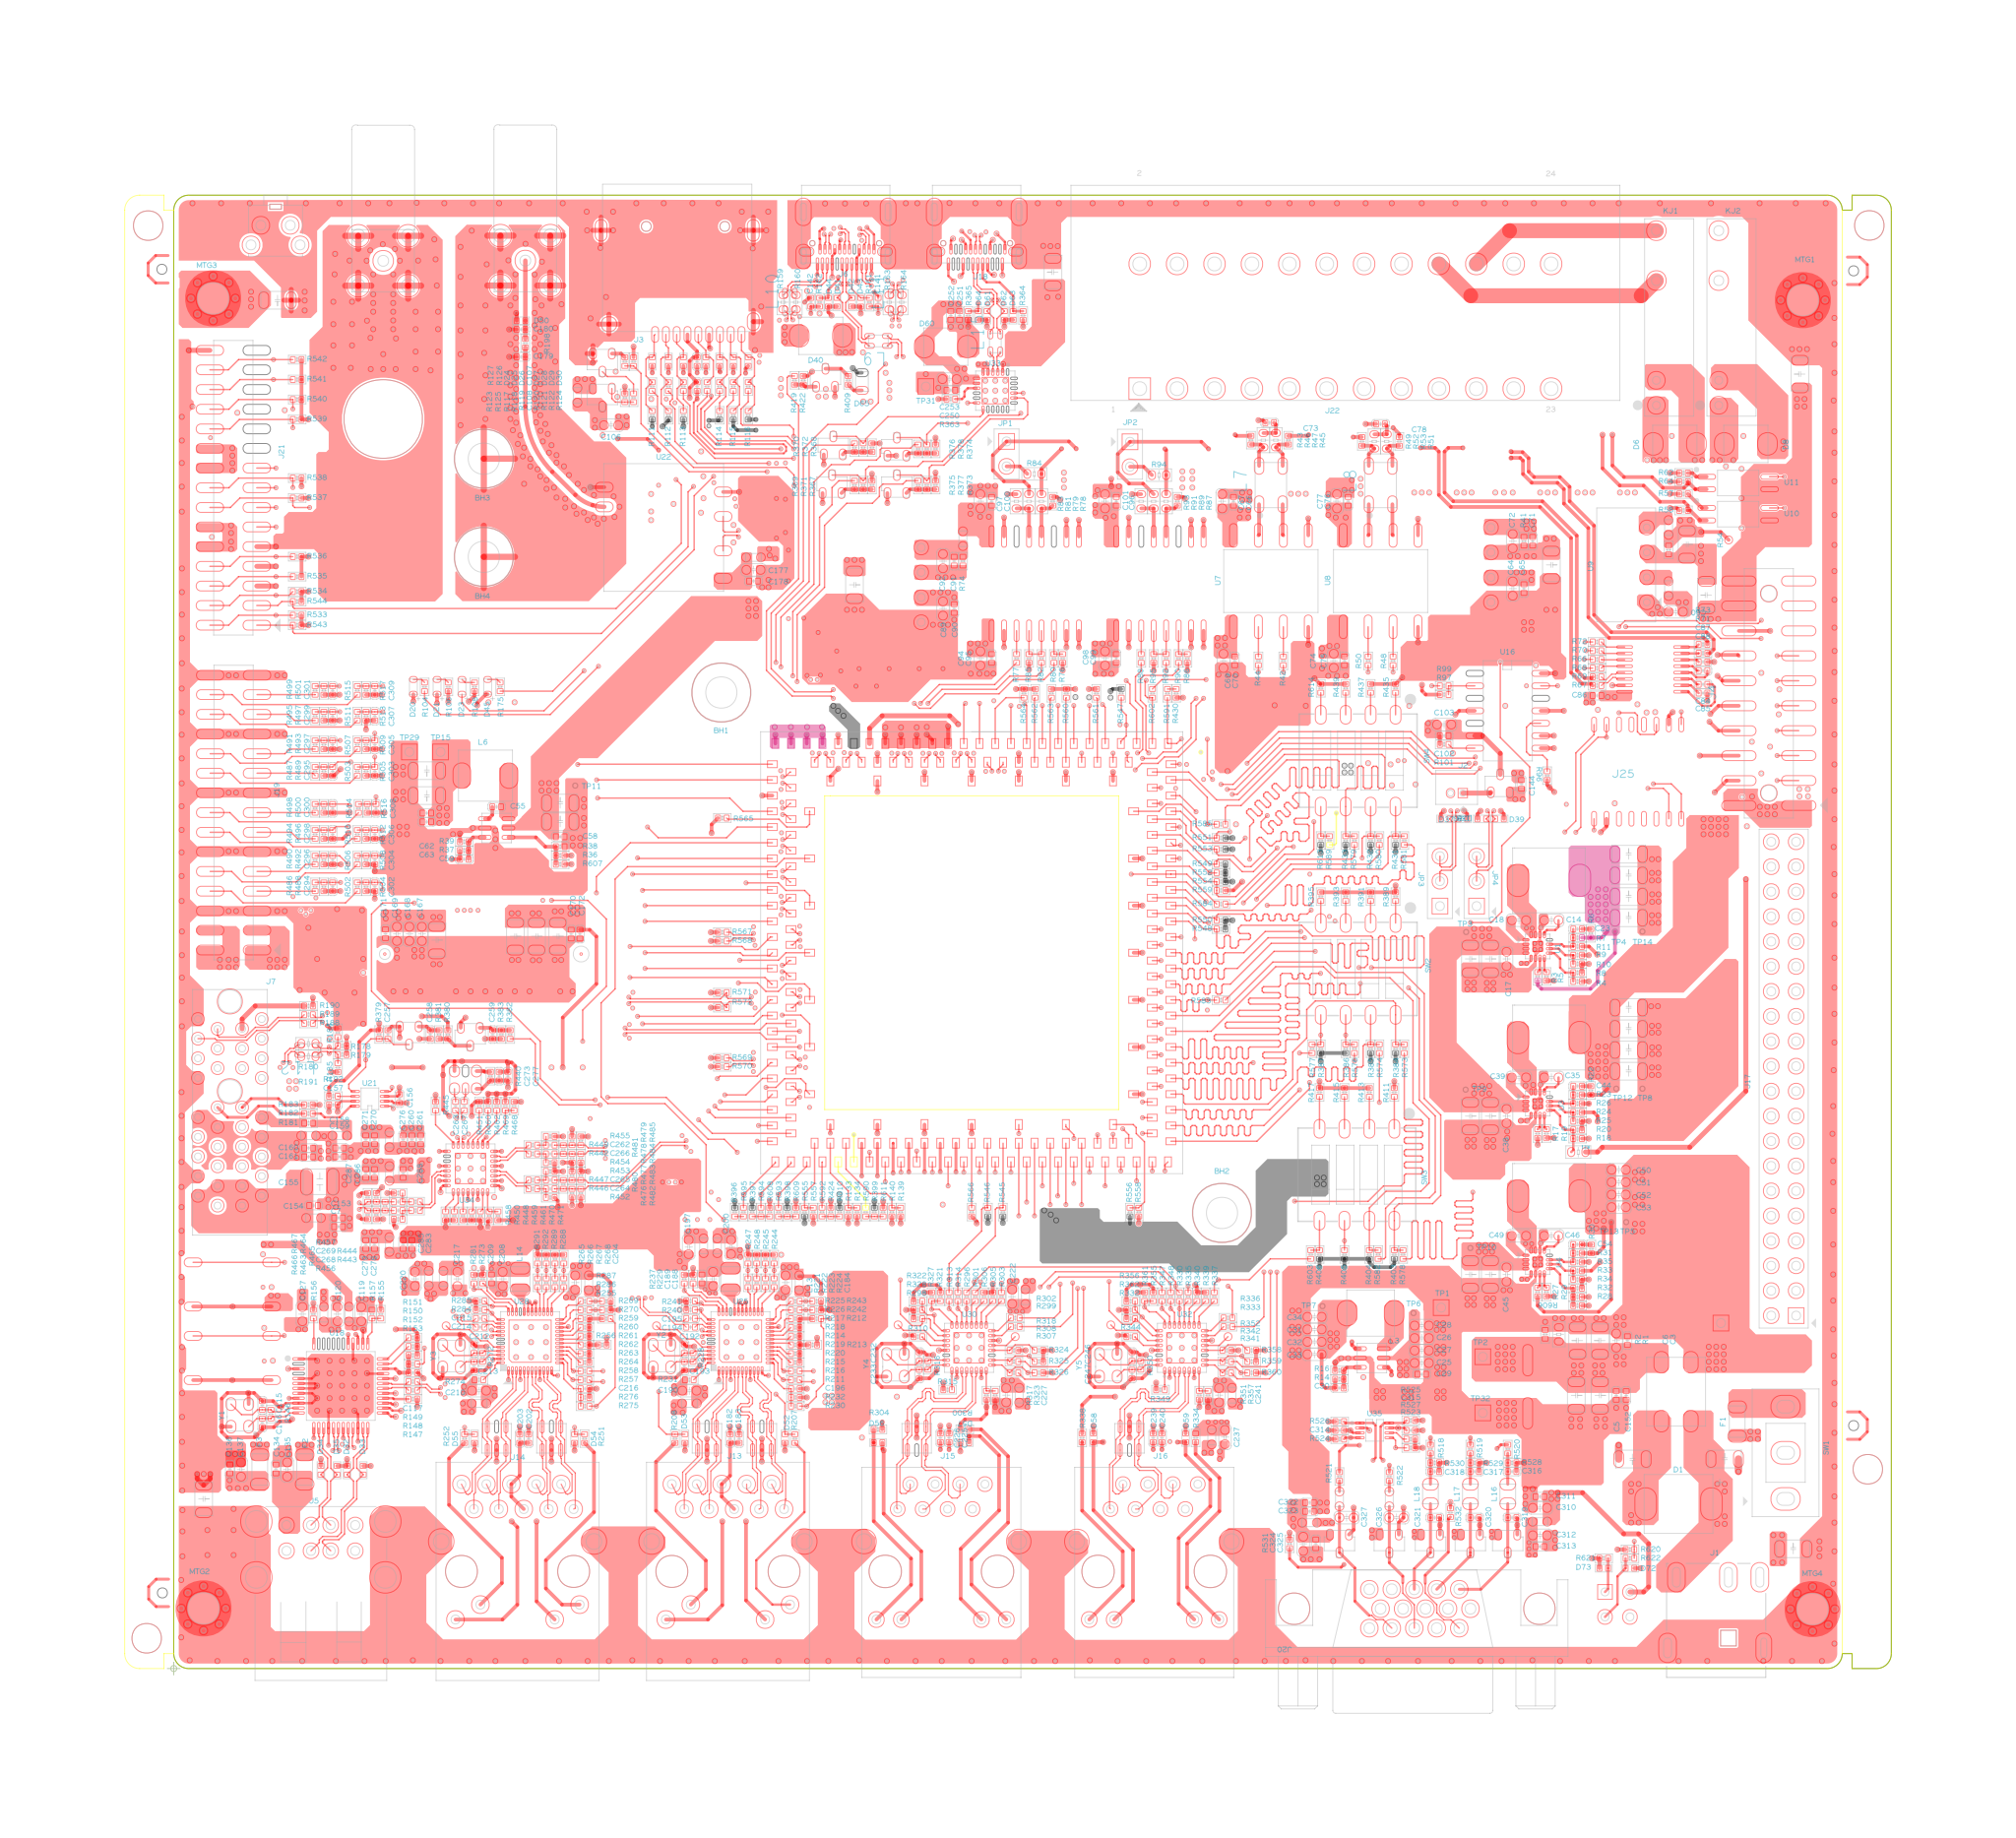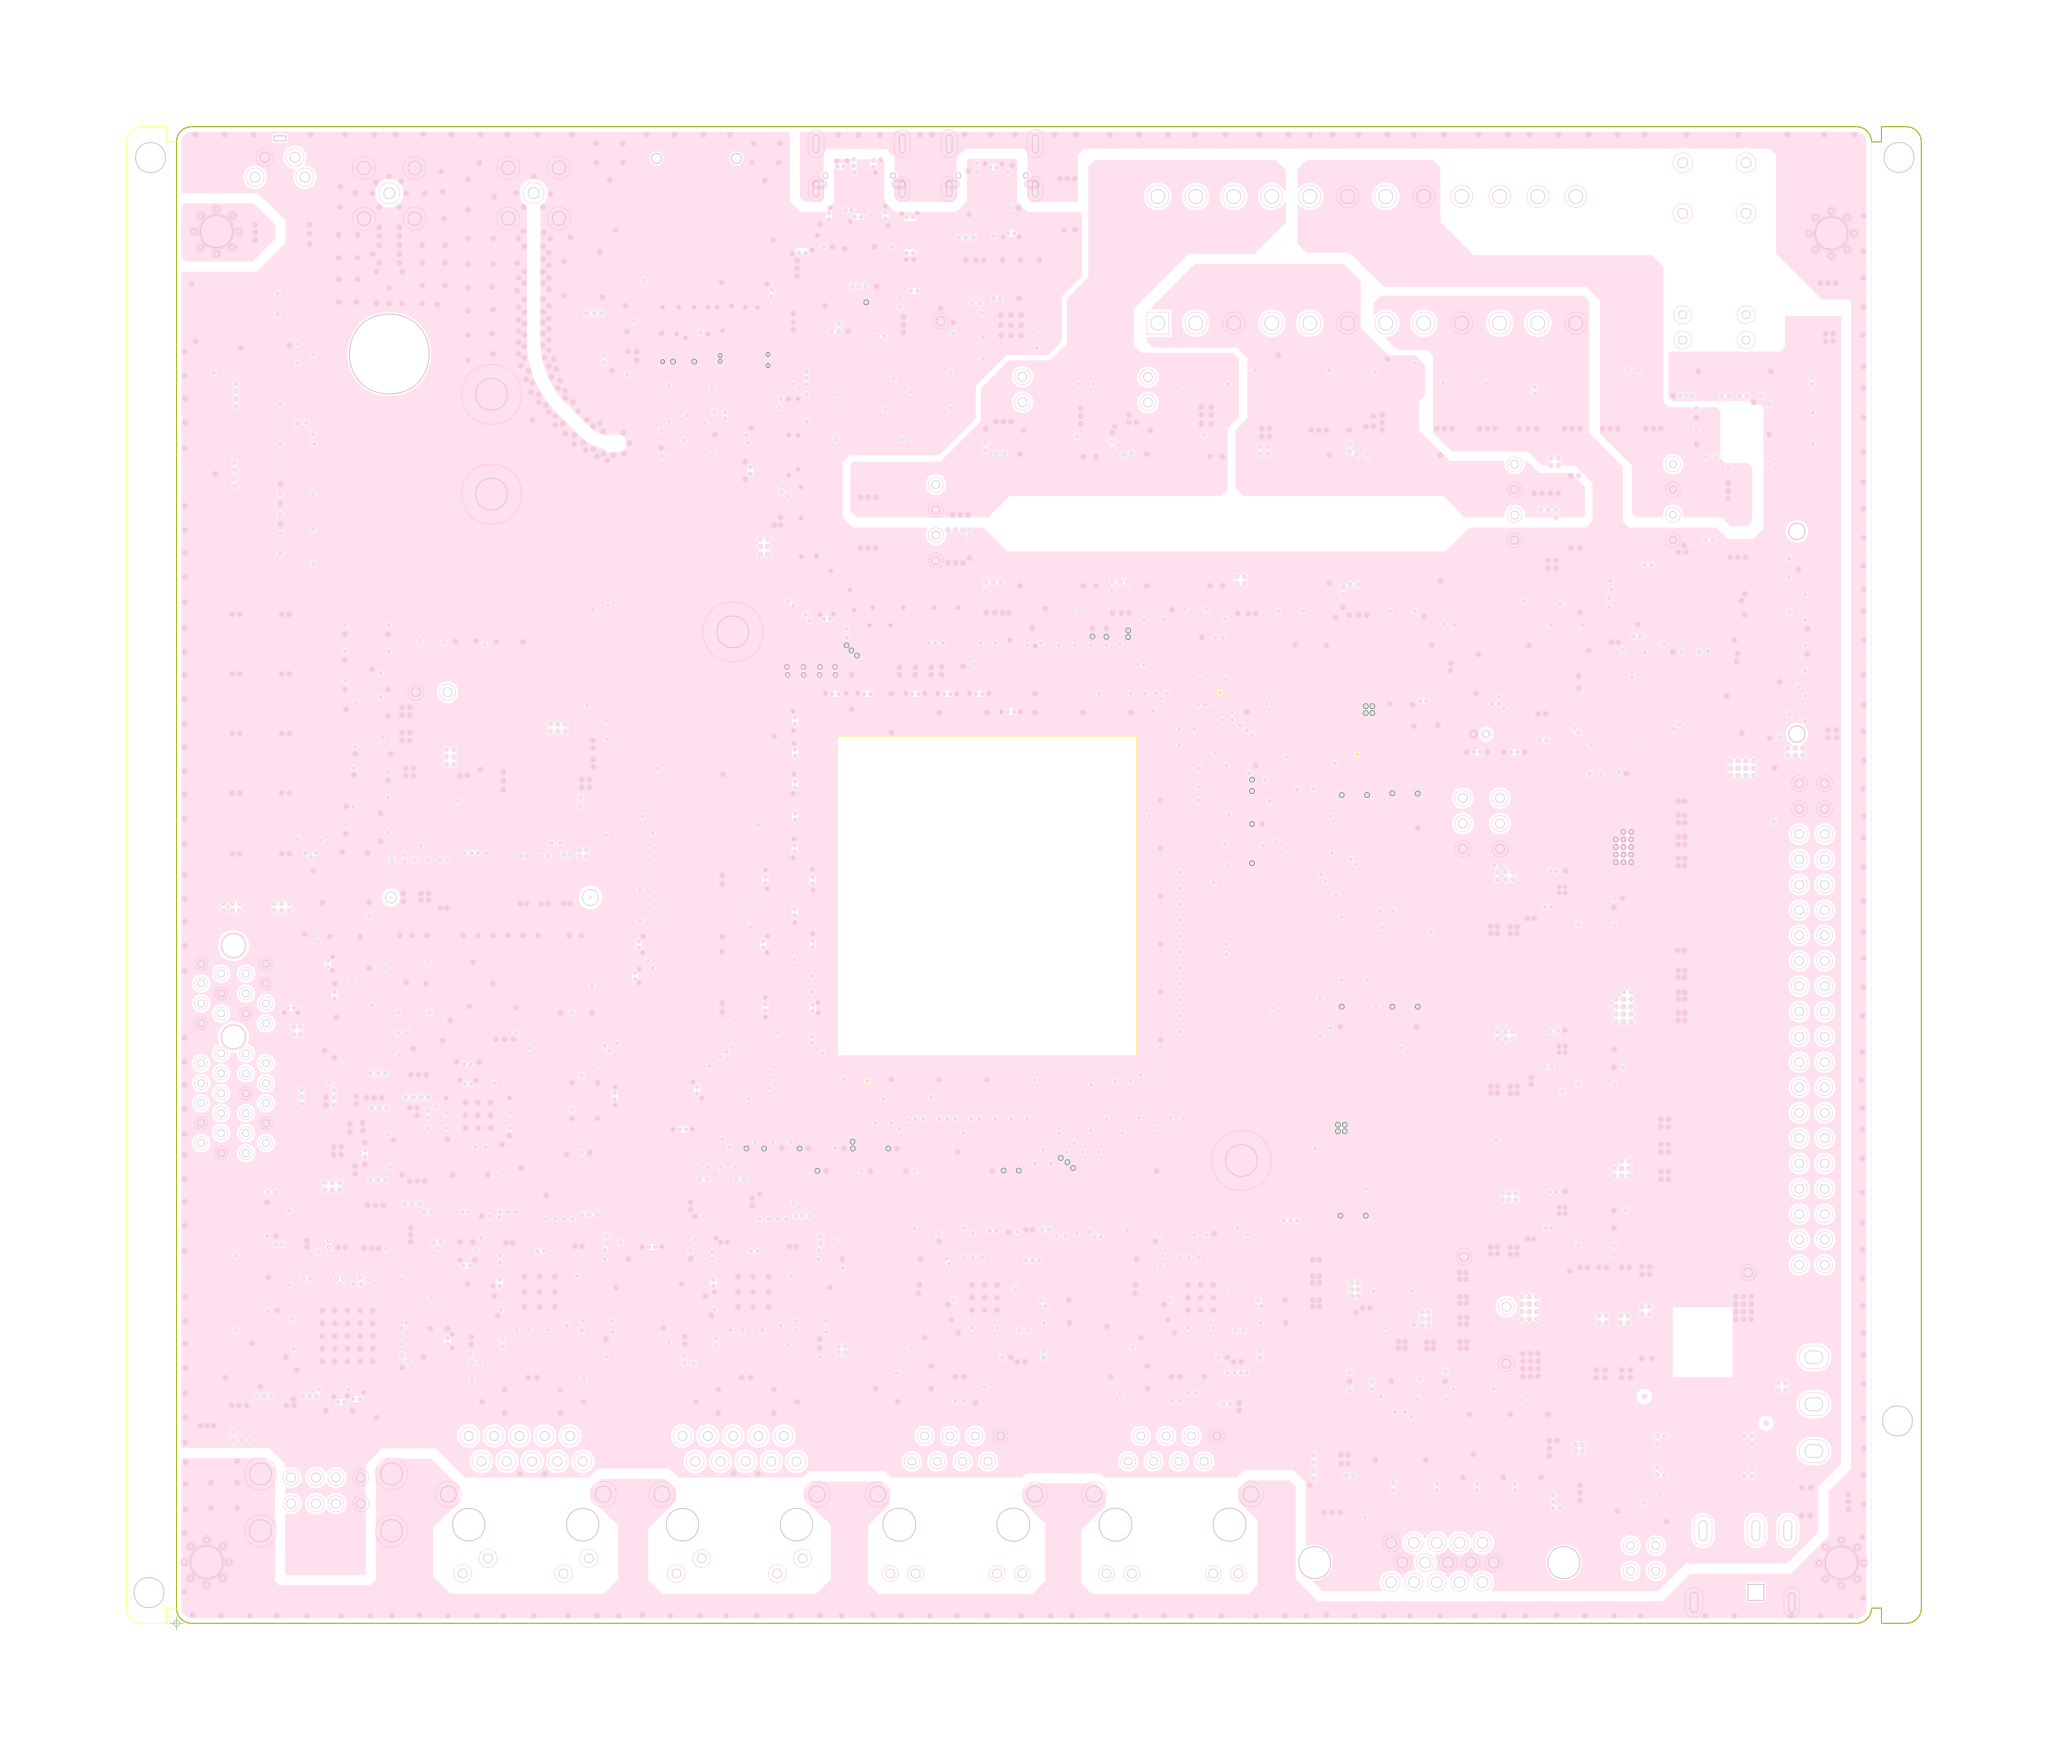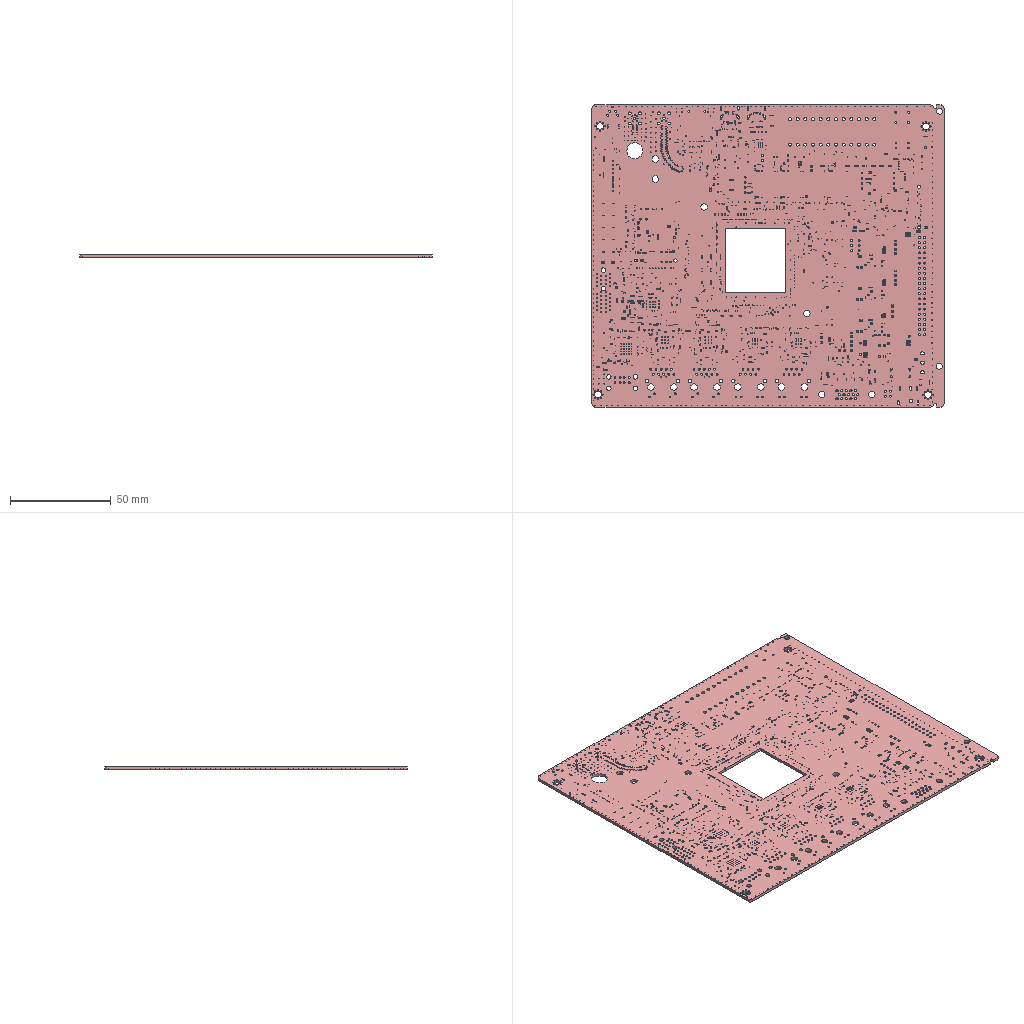Circuit board layout | Cadence Allegro | box 175 x 150 x 1.5 mm
Layer stack:
# Cadence Allegro layer stack of  (unit mm; from the constraint file cross-section; dielectric type: 0 not recorded (Allegro does not mark core vs prepreg), 3 surface material)
index,name,kind,layer,copper_thickness_mm,dielectric_type,dielectric_thickness_mm,dielectric_material,dielectric_constant
0,Top Surface,other,,,,,,
1,TOP,copper,TOP,0.036,,,,
2,Dielectric1,dielectric,,,0,0.0911,FR-4,3.95
3,GND02,copper,GND02,0.03,,,,
4,Dielectric2,dielectric,,,0,0.127,FR-4,3.95
5,ART03,copper,ART03,0.03,,,,
6,Dielectric3,dielectric,,,0,0.927,FR-4,4.5
7,POWER04,copper,POWER04,0.03,,,,
8,Dielectric4,dielectric,,,0,0.127,FR-4,4.5
9,GND05,copper,GND05,0.03,,,,
10,Dielectric5,dielectric,,,0,0.0911,FR-4,4.5
11,BOTTOM,copper,BOTTOM,0.036,,,,
12,Bottom Surface,other,,,,,,
# drill layer pairs: low layer,high layer
drill_pair,TOP,BOTTOM
Part placement, first 442 of 1160 lines:
REFDES,COMP_VALUE,SYM_NAME,SYM_X,SYM_Y,SYM_ROTATE,SYM_MIRROR
BH1,TP,MH236-125T,2196.06,3913.31,0.000,NO
BH2,TP,MH236-125T,4203.94,1826.69,0.000,NO
BH3,TP,MH236-125T,1243.50,4850.83,0.000,NO
BH4,TP,MH236-125T,1243.50,4457.16,0.000,NO
C1,22uF/12/25V,C1206,6035.00,625.00,180.000,YES
C2,22uF/12/25V,C1206,6035.00,715.00,180.000,YES
C3,100nF/4/50V,C0402,5830.00,1315.00,90.000,NO
C4,100uF/6x7/25V,CE6X6,5430.00,1130.00,180.000,NO
C5,100nF/4/50V,C0402,5785.00,1095.00,270.000,NO
C6,1uF/6/25V,C0603,5785.00,1315.00,90.000,NO
C7,100nF/4/50V,C0402,660.71,1771.56,0.000,NO
C8,DNP/C1206,C1206,5720.00,1095.00,270.000,NO
C9,DNP/C1206,C1206,5630.00,1315.00,90.000,NO
C10,22uF/12/25V,C1206,5200.08,2214.92,270.000,NO
C11,22uF/12/25V,C1206,5280.08,2214.92,270.000,NO
C12,DNP/C1206,C1206,5850.00,840.00,180.000,NO
C13,DNP/C1206,C1206,6220.00,840.00,0.000,NO
C14,2.2uF/6/16V,C0603,5525.08,3000.08,0.000,NO
C15,22uF/12/25V,C1206,5625.00,1095.00,270.000,NO
C16,22uF/12/25V,C1206,5720.00,1315.00,90.000,NO
C17,100nF/6/50V,C0603,5345.08,2845.08,270.000,NO
C18,100nF/6/50V,C0603,5395.08,3000.08,0.000,NO
C19,22uF/12/25V,C1206,5835.08,3265.08,0.000,NO
C20,22uF/12/25V,C1206,5835.08,3180.08,0.000,NO
C21,22uF/12/25V,C1206,5835.08,3095.08,0.000,NO
C22,22uF/12/25V,C1206,5835.08,3010.08,0.000,NO
C23,68pF/4/50V,C0402,5630.08,2965.08,180.000,NO
C24,100nF/6/50V,C0603,4805.00,1285.00,180.000,YES
C25,10uF/6/16V,C0603,5005.00,1225.00,0.000,NO
C26,10uF/6/16V,C0603,5005.00,1325.00,0.000,NO
C27,10uF/6/16V,C0603,5005.00,1275.00,0.000,NO
C28,10uF/6/16V,C0603,5005.00,1375.00,0.000,NO
C29,100nF/4/50V,C0402,5005.00,1180.00,0.000,NO
C30,68pF/4/50V,C0402,4675.00,1125.00,0.000,NO
C31,22uF/6/6.3V,C0603,4575.00,1360.00,180.000,NO
C32,22uF/6/6.3V,C0603,4575.00,1310.00,180.000,NO
C33,47uF/6/6.3V,C0603,4575.00,1260.00,180.000,NO
C34,47uF/6/6.3V,C0603,4575.00,1410.00,180.000,NO
C35,2.2uF/6/16V,C0603,5525.08,2369.92,0.000,NO
C36,22uF/12/25V,C1206,5280.08,2845.08,270.000,NO
C37,22uF/12/25V,C1206,5200.08,2845.08,270.000,NO
C38,100nF/6/50V,C0603,5345.08,2214.92,270.000,NO
C39,100nF/6/50V,C0603,5395.08,2369.92,0.000,NO
C40,22uF/12/25V,C1206,5279.92,1579.92,270.000,NO
C41,22uF/12/25V,C1206,5835.08,2479.92,0.000,NO
C42,22uF/12/25V,C1206,5835.08,2394.92,0.000,NO
C43,22uF/12/25V,C1206,5835.08,2649.92,0.000,NO
C44,68pF/4/50V,C0402,5630.08,2334.92,180.000,NO
C45,100nF/6/50V,C0603,5344.92,1579.92,270.000,NO
C46,2.2uF/6/16V,C0603,5524.92,1734.92,0.000,NO
C47,22uF/12/25V,C1206,5199.92,1579.92,270.000,NO
C48,22uF/12/25V,C1206,5835.08,2564.92,0.000,NO
C49,100nF/6/50V,C0603,5394.92,1734.92,0.000,NO
C50,22uF/6/6.3V,C0603,5795.00,2000.00,0.000,NO
C51,22uF/6/6.3V,C0603,5795.00,1950.00,0.000,NO
C52,22uF/6/6.3V,C0603,5795.00,1900.00,0.000,NO
C53,22uF/6/6.3V,C0603,5795.00,1850.00,0.000,NO
C54,68pF/4/50V,C0402,5629.92,1699.92,180.000,NO
C55,100nF/4/50V,C0402,1295.00,3455.00,0.000,NO
C56,22uF/12/25V,C1206,1550.00,3470.00,0.000,NO
C57,22uF/12/25V,C1206,1550.00,3395.00,0.000,NO
C58,100nF/4/50V,C0402,1550.00,3335.00,0.000,NO
C59,1uF/4/50V,C0402,1165.00,3245.00,0.000,NO
C60,DNP,C1206,1015.00,3500.00,180.000,NO
C61,22uF/12/25V,C1206,1015.00,3600.00,180.000,NO
C62,100nF/4/50V,C0402,1015.00,3430.00,180.000,NO
C63,100nF/4/50V,C0402,1015.00,3395.00,180.000,NO
C64,10uF/6/16V,C0603,5370.00,4329.95,270.000,NO
C65,100nF/4/50V,C0402,5415.00,4329.95,270.000,NO
C66,100nF/4/50V,C0402,4250.00,4680.00,90.000,NO
C67,10uF/6/16V,C0603,4205.00,4680.00,90.000,NO
C68,DNP/C1206,C1206,5525.00,4424.95,270.000,NO
C69,10uF/6/10V,C0603,4210.00,4040.00,270.000,NO
C70,100nF/4/50V,C0402,4255.00,4040.00,270.000,NO
C71,100nF/4/50V,C0402,5450.00,4519.95,270.000,NO
C72,10uF/6/10V,C0603,5370.00,4519.95,270.000,NO
C73,68pF/4/50V,C0402,4395.00,4995.00,180.000,NO
C74,10uF/6/10V,C0603,4652.24,4040.41,270.000,NO
C75,100nF/4/50V,C0402,4695.00,4040.00,270.000,NO
C76,100nF/4/50V,C0402,4710.00,4680.00,90.000,NO
C77,10uF/6/10V,C0603,4665.00,4680.00,90.000,NO
C78,68pF/4/50V,C0402,4840.00,4990.00,180.000,NO
C79,22uF/12/25V,C1206,6069.00,4507.00,270.000,NO
C80,10uF/6/16V,C0603,6024.00,4237.00,180.000,NO
C81,DNP/C1206,C1206,6147.00,4304.00,90.000,NO
C82,10nF/4/50V,C0402,6305.00,4657.69,0.000,YES
C83,10nF/4/50V,C0402,6305.00,4732.31,0.000,YES
C84,100nF/4/50V,C0402,6133.00,3946.00,180.000,NO
C85,100nF/4/50V,C0402,6133.00,3911.00,180.000,NO
C86,100nF/4/50V,C0402,5708.00,3901.00,180.000,NO
C87,100nF/4/50V,C0402,6133.00,4036.00,180.000,NO
C88,100nF/4/50V,C0402,6133.00,4001.00,180.000,NO
C89,10uF/6/16V,C0603,3085.00,4249.95,270.000,NO
C90,100nF/4/50V,C0402,3130.00,4249.95,270.000,NO
C91,100nF/4/50V,C0402,3130.00,4439.95,270.000,NO
C92,10uF/6/16V,C0603,3085.00,4439.95,270.000,NO
C93,DNP/C1206,C1206,2730.00,4344.95,270.000,NO
C94,10uF/6/16V,C0603,3235.00,4050.00,270.000,NO
C95,100nF/4/50V,C0402,3280.00,4050.00,270.000,NO
C96,100nF/4/50V,C0402,3780.00,4680.00,90.000,NO
C97,10uF/6/16V,C0603,3235.00,4680.00,90.000,NO
C98,10uF/6/16V,C0603,3735.00,4050.00,270.000,NO
C99,100nF/4/50V,C0402,3780.00,4050.00,270.000,NO
C100,100nF/4/50V,C0402,3280.00,4680.00,90.000,NO
C101,10uF/6/16V,C0603,3735.00,4680.00,90.000,NO
C102,100nF/4/50V,C0402,5095.00,3740.00,180.000,NO
C103,10uF/6/16V,C0603,5095.00,3785.00,180.000,NO
C104,100nF/4/50V,C0402,375.00,1560.00,180.000,YES
C105,100nF/4/50V,C0402,380.00,1265.00,180.000,YES
C106,10uF/6/16V,C0603,1754.00,4985.00,0.000,NO
C107,1uF/4/6.3V,C0402,2099.00,5240.00,270.000,NO
C108,100nF/4/50V,C0402,2099.00,5140.00,270.000,NO
C109,10uF/6/16V,C0603,6495.96,3457.99,180.000,YES
C110,100nF/4/50V,C0402,6307.04,3458.01,0.000,YES
C111,18pF/4/50V,C0402,6401.99,3843.04,90.000,YES
C112,18pF/4/50V,C0402,6401.99,3943.04,90.000,YES
C113,18pF/4/50V,C0402,6366.99,3743.04,90.000,YES
C114,100nF/4/50V,C0402,5924.00,3801.00,0.000,YES
C115,DNP,C0402,355.00,1055.00,90.000,NO
C116,DNP,C0402,355.00,985.00,270.000,NO
C117,DNP,C0402,959.00,1186.00,0.000,NO
C118,100nF/4/50V,C0402,775.00,1295.00,90.000,YES
C119,10uF/6/10V,C0603,752.00,1421.00,90.000,NO
C120,10uF/6/10V,C0603,657.00,1421.00,90.000,NO
C121,100nF/4/50V,C0402,560.00,975.00,270.000,YES
C122,100nF/4/50V,C0402,680.00,970.00,270.000,YES
C123,100nF/4/50V,C0402,835.00,1065.00,0.000,YES
C124,100nF/4/50V,C0402,835.00,1165.00,0.000,YES
C125,100nF/4/50V,C0402,700.00,1295.00,90.000,YES
C126,100nF/4/50V,C0402,740.00,1295.00,90.000,YES
C127,10uF/6/10V,C0603,516.00,1421.00,90.000,NO
C128,100nF/4/50V,C0402,835.00,1100.00,0.000,YES
C129,100nF/4/50V,C0402,505.00,1165.00,180.000,YES
C130,100nF/4/50V,C0402,835.00,1030.00,0.000,YES
C131,100nF/4/50V,C0402,510.00,1085.00,180.000,YES
C132,100nF/4/50V,C0402,505.00,1200.00,180.000,YES
C133,100nF/4/50V,C0402,510.00,1050.00,180.000,YES
C134,100nF/4/50V,C0402,410.00,800.00,90.000,NO
C135,10uF/6/10V,C0603,455.00,798.00,90.000,NO
C136,100nF/4/50V,C0402,225.00,800.00,90.000,NO
C137,10uF/6/10V,C0603,270.00,798.00,90.000,NO
C139,100nF/4/50V,C0402,2625.00,5478.13,90.000,YES
C140,10pF/4/50V,C0402,2555.00,5478.13,90.000,YES
C141,1nF/4/50V,C0402,2825.00,5478.13,90.000,NO
C142,1nF/4/50V,C0402,2555.00,5478.13,90.000,NO
C144,100nF/4/50V,C0402,5405.00,3545.00,90.000,NO
C145,100nF/4/50V,C0402,2590.00,5478.13,90.000,YES
C146,10uF/6/16V,C0603,2809.88,5115.00,180.000,YES
C147,100nF/4/50V,C0402,2809.88,5160.00,180.000,YES
C148,4.7uF/6/16V,C0603,2509.88,5155.00,0.000,YES
C149,100nF/4/50V,C0402,2755.00,5478.13,90.000,YES
C150,100nF/4/50V,C0402,2790.00,5478.13,90.000,YES
C151,10uF/6/16V,C0603,2509.88,5105.00,0.000,YES
C152,100nF/4/50V,C0402,5825.00,1095.00,270.000,NO
C153,100nF/4/50V,C0402,660.71,1806.56,0.000,NO
C154,100nF/4/50V,C0402,560.71,1856.56,0.000,NO
C155,10uF/1210/50V,C1210,585.71,1951.56,0.000,NO
C156,100nF/4/50V,C0402,905.00,2285.00,270.000,NO
C157,100nF/4/50V,C0402,640.00,2260.00,180.000,NO
C158,100nF/4/50V,C0402,665.00,2087.00,0.000,NO
C159,100nF/4/50V,C0402,665.00,2052.00,0.000,NO
C160,100nF/4/50V,C0402,540.71,2086.56,0.000,NO
C161,100nF/4/50V,C0402,540.71,2051.56,0.000,NO
C162,33pF/4/50V,C0402,1720.00,5020.00,90.000,YES
C163,100nF/4/50V,C0402,1720.00,5140.00,90.000,YES
C164,100uF/12/6.3V,C1206,1455.00,2935.64,270.000,NO
C165,100uF/12/6.3V,C1206,1540.00,2935.64,270.000,NO
C166,100uF/12/6.3V,C1206,1370.00,2935.64,270.000,NO
C167,10uF/6/16V,C0603,995.00,2945.64,270.000,NO
C168,10uF/6/16V,C0603,945.00,2945.64,270.000,NO
C169,1uF/6/16V,C0603,895.00,2945.64,270.000,NO
C170,100nF/4/50V,C0402,1594.00,2944.64,270.000,NO
C171,33pF/4/50V,C0402,849.00,2946.00,270.000,NO
C172,10nF/4/50V,C0402,1629.00,2944.64,270.000,NO
C173,33pF/4/50V,C0402,1910.00,5030.00,270.000,YES
C174,33pF/4/50V,C0402,2020.00,5030.00,270.000,YES
C175,33pF/4/50V,C0402,1975.00,5030.00,270.000,YES
C176,100uF/12/6.3V,C1206,1055.00,2920.64,270.000,NO
C177,10uF/6/16V,C0603,2325.00,4405.00,0.000,NO
C178,100nF/4/50V,C0402,2325.00,4360.00,0.000,NO
C179,DNP,C0402,1392.68,5259.00,180.000,NO
C180,DNP,C0402,1392.68,5369.00,180.000,NO
C181,10nF/4/50V,C0402,1515.00,2455.00,90.000,YES
C182,100nF/4/50V,C0402,2231.13,922.00,90.000,NO
C183,100nF/4/50V,C0402,2267.13,922.00,90.000,NO
C184,4.7uF/6/16V,C0603,2453.74,1547.61,270.000,NO
C185,100nF/4/50V,C0402,2245.13,1431.00,0.000,YES
C186,100nF/4/50V,C0402,2316.13,1431.00,180.000,YES
C188,4.7uF/6/16V,C0603,2163.13,1562.00,270.000,NO
C189,100nF/4/50V,C0402,2118.13,1562.00,270.000,NO
C190,10uF/6/16V,C0603,2068.13,1114.00,180.000,NO
C191,100nF/4/50V,C0402,2202.13,1195.00,180.000,YES
C192,33pF/4/50V,C0402,2047.74,1282.61,90.000,NO
C193,33pF/4/50V,C0402,2047.74,1212.61,270.000,NO
C194,10nF/4/50V,C0402,2072.74,1368.61,0.000,NO
C195,10nF/4/50V,C0402,2072.74,1403.61,0.000,NO
C196,100nF/4/50V,C0402,2493.13,1122.00,0.000,NO
C197,4.7uF/6/16V,C0603,2065.00,1690.00,270.000,NO
C198,100nF/4/50V,C0402,2272.13,1195.00,180.000,YES
C199,100nF/4/50V,C0402,2156.13,1242.00,270.000,YES
C200,10uF/6/16V,C0603,2235.00,1690.00,270.000,NO
C201,100nF/4/50V,C0402,2392.13,1351.00,90.000,YES
C202,100nF/4/50V,C0402,1423.33,922.00,90.000,NO
C203,100nF/4/50V,C0402,1387.33,922.00,90.000,NO
C204,4.7uF/6/16V,C0603,1609.94,1547.61,270.000,NO
C205,100nF/4/50V,C0402,1401.33,1431.00,0.000,YES
C206,100nF/4/50V,C0402,1472.33,1431.00,180.000,YES
C208,4.7uF/6/16V,C0603,1319.33,1562.00,270.000,NO
C209,100nF/4/50V,C0402,1274.33,1562.00,270.000,NO
C210,10uF/6/16V,C0603,1224.33,1114.00,180.000,NO
C211,100nF/4/50V,C0402,1358.33,1195.00,180.000,YES
C212,33pF/4/50V,C0402,1203.94,1282.61,90.000,NO
C213,33pF/4/50V,C0402,1203.94,1212.61,270.000,NO
C214,10nF/4/50V,C0402,1228.94,1368.61,0.000,NO
C215,10nF/4/50V,C0402,1228.94,1403.61,0.000,NO
C216,100nF/4/50V,C0402,1649.33,1122.00,0.000,NO
C217,4.7uF/6/16V,C0603,1137.54,1562.00,270.000,NO
C218,100nF/4/50V,C0402,1310.89,1240.11,270.000,YES
C219,100nF/4/50V,C0402,1428.33,1195.00,180.000,YES
C220,10uF/6/16V,C0603,967.54,1562.00,270.000,NO
C221,100nF/4/50V,C0402,1548.33,1351.00,90.000,YES
C222,10uF/6/16V,C0603,3362.57,1490.80,90.000,NO
C223,100nF/4/50V,C0402,3280.57,1296.80,90.000,YES
C224,100nF/4/50V,C0402,3249.57,1490.80,270.000,YES
C225,100nF/4/50V,C0402,3109.57,925.00,90.000,NO
C226,100nF/4/50V,C0402,3074.57,925.00,90.000,NO
C227,10uF/6/16V,C0603,3338.57,1095.80,270.000,NO
C228,100nF/4/50V,C0402,3257.57,1193.80,180.000,YES
C230,1uF/4/6.3V,C0402,3187.57,1193.80,180.000,YES
C231,100nF/4/50V,C0402,3117.57,1193.80,0.000,YES
C232,33pF/4/50V,C0402,2989.57,1250.80,90.000,NO
C233,33pF/4/50V,C0402,2989.57,1180.80,270.000,NO
C234,1uF/4/6.3V,C0402,3098.57,1256.80,90.000,YES
C235,100nF/4/50V,C0402,3098.57,1326.80,270.000,YES
C236,100nF/4/50V,C0402,4103.11,1490.80,270.000,YES
C237,10uF/6/16V,C0603,4215.89,928.20,270.000,NO
C238,100nF/4/50V,C0402,4134.11,1296.80,90.000,YES
C239,100nF/4/50V,C0402,3928.11,925.00,90.000,NO
C240,100nF/4/50V,C0402,3963.11,925.00,90.000,NO
C241,10uF/6/16V,C0603,4192.11,1095.80,270.000,NO
C242,100nF/4/50V,C0402,4111.11,1193.80,180.000,YES
C244,1uF/4/6.3V,C0402,4041.11,1193.80,180.000,YES
C245,100nF/4/50V,C0402,3971.11,1193.80,0.000,YES
C246,33pF/4/50V,C0402,3843.11,1250.80,90.000,NO
C247,33pF/4/50V,C0402,3843.11,1180.80,270.000,NO
C248,1uF/4/6.3V,C0402,3952.11,1256.80,90.000,YES
C249,100nF/4/50V,C0402,3952.11,1326.80,270.000,YES
C250,100nF/4/50V,C0402,3116.33,5125.00,180.000,NO
C251,10pF/4/50V,C0402,3151.33,5425.00,270.000,NO
C252,100nF/4/50V,C0402,3116.33,5425.00,270.000,NO
C253,10uF/6/16V,C0603,3111.33,5170.00,180.000,NO
C254,DNP,C0603,3220.17,5150.00,90.000,YES
C255,100nF/4/50V,C0402,3280.17,5200.00,180.000,YES
C256,0,C1206,3526.00,5599.00,90.000,NO
C257,100nF/4/50V,C0402,859.00,2542.00,90.000,NO
C258,100nF/4/50V,C0402,1029.00,2542.00,270.000,NO
C259,10nF/4/50V,C0402,1279.00,2542.00,270.000,NO
C260,10uF/6/16V,C0402,955.00,2120.00,90.000,NO
C261,100nF/4/50V,C0402,990.00,2120.00,90.000,NO
C262,100nF/4/50V,C0402,1510.00,2098.45,180.000,NO
C263,100nF/4/50V,C0402,1130.00,2255.00,270.000,NO
C264,100nF/4/50V,C0402,1510.00,1923.45,180.000,NO
C265,100nF/4/50V,C0402,1510.00,1958.45,180.000,NO
C266,100nF/4/50V,C0402,1510.00,2063.45,180.000,NO
C267,100nF/4/50V,C0402,1165.00,2255.00,270.000,NO
C268,100nF/4/50V,C0402,900.00,1836.43,0.000,NO
C269,100nF/4/50V,C0402,900.00,1871.43,0.000,NO
C270,10uF/4/6.3V,C0402,805.00,2120.00,270.000,NO
C271,100nF/4/50V,C0402,770.00,2120.00,270.000,NO
C272,100nF/4/50V,C0402,920.00,2120.00,270.000,YES
C273,10uF/4/6.3V,C0402,1305.00,2375.00,90.000,NO
C274,10uF/4/6.3V,C0402,990.00,2120.00,270.000,YES
C275,100nF/4/50V,C0402,955.00,2120.00,270.000,YES
C276,100nF/4/50V,C0402,920.00,2120.00,90.000,NO
C277,100nF/4/50V,C0402,1340.00,2375.00,90.000,NO
C278,10uF/4/6.3V,C0402,805.00,1700.00,270.000,NO
C279,100nF/4/50V,C0402,770.00,1700.00,270.000,NO
C280,100nF/4/50V,C0402,1220.00,2100.00,0.000,YES
C281,10uF/4/6.3V,C0402,920.00,1700.00,270.000,YES
C282,10uF/4/6.3V,C0402,1155.00,1910.00,0.000,YES
C283,100nF/4/50V,C0402,955.00,1700.00,90.000,NO
C284,100nF/4/50V,C0402,955.00,1700.00,270.000,YES
C285,100nF/4/50V,C0402,920.00,1700.00,90.000,NO
C286,10uF/4/6.3V,C0402,805.00,1985.00,270.000,NO
C287,100nF/4/50V,C0402,770.00,1985.00,270.000,NO
C288,100nF/4/50V,C0402,920.00,1985.00,90.000,NO
C289,10uF/4/6.3V,C0402,1240.00,1910.00,180.000,YES
C290,10uF/4/6.3V,C0402,1285.00,2050.00,270.000,YES
C291,100nF/4/50V,C0402,1095.00,2040.00,270.000,YES
C292,100nF/4/50V,C0402,1095.00,1945.00,90.000,YES
C293,100nF/4/50V,C0402,1285.00,1960.00,90.000,YES
C294,10nF/4/50V,C0402,637.10,3134.47,270.000,NO
C295,10nF/4/50V,C0402,637.10,3597.47,270.000,NO
C296,10nF/4/50V,C0402,637.10,3241.47,270.000,NO
C297,10nF/4/50V,C0402,637.10,3703.69,270.000,NO
C298,10nF/4/50V,C0402,637.10,3344.47,270.000,NO
C299,10nF/4/50V,C0402,637.10,3818.69,270.000,NO
C300,10nF/4/50V,C0402,637.10,3448.69,270.000,NO
C301,10nF/4/50V,C0402,637.10,3921.69,270.000,NO
C302,10nF/4/50V,C0402,806.10,3134.47,270.000,NO
C303,10nF/4/50V,C0402,806.10,3597.47,270.000,NO
C304,10nF/4/50V,C0402,806.10,3241.47,270.000,NO
C305,10nF/4/50V,C0402,806.10,3703.69,270.000,NO
C306,10nF/4/50V,C0402,806.10,3344.47,270.000,NO
C307,10nF/4/50V,C0402,806.10,3818.69,270.000,NO
C308,10nF/4/50V,C0402,811.10,3448.69,270.000,NO
C309,10nF/4/50V,C0402,806.10,3921.69,270.000,NO
C310,10uF/6/16V,C0603,5479.00,644.00,180.000,NO
C311,100nF/4/50V,C0402,5479.00,689.00,180.000,NO
C312,10uF/6/16V,C0603,5479.00,534.00,0.000,NO
C313,100nF/4/50V,C0402,5479.00,489.00,0.000,NO
C314,100nF/4/50V,C0402,4676.00,955.00,180.000,NO
C315,100nF/4/50V,C0402,4961.00,955.00,0.000,NO
C316,10pF/4/50V,C0402,5367.32,790.00,0.000,NO
C317,10pF/4/50V,C0402,5217.32,790.00,0.000,NO
C318,10pF/4/50V,C0402,5057.32,790.00,0.000,NO
C319,10pF/4/50V,C0402,5367.32,605.00,0.000,NO
C320,10pF/4/50V,C0402,5217.32,605.00,0.000,NO
C321,10pF/4/50V,C0402,5057.32,605.00,0.000,NO
C322,10uF/6/16V,C0402,4555.00,665.00,0.000,NO
C323,100nF/4/50V,C0402,4555.00,630.00,0.000,NO
C324,10uF/6/16V,C0603,4530.00,500.00,270.000,NO
C325,100nF/4/50V,C0402,4580.00,500.00,270.000,NO
C326,470pF/6/50V,C0603,4903.51,605.00,0.000,NO
C327,470pF/6/50V,C0603,4703.51,605.00,0.000,NO
C328,0,C1206,416.00,5486.00,180.000,NO
C329,0,C1206,6522.00,5190.00,90.000,NO
C330,0,C1206,6495.00,480.00,0.000,NO
C331,0,C1206,120.00,680.00,270.000,NO
C332,100nF/4/50V,C0402,2390.00,1245.00,270.000,YES
C333,100nF/4/50V,C0402,2345.00,1195.00,180.000,YES
C334,100nF/4/50V,C0402,1545.00,1247.00,270.000,YES
C335,100nF/4/50V,C0402,1500.00,1195.00,180.000,YES
C336,100nF/4/50V,C0402,390.00,5080.00,180.000,YES
D1,SMCJ15CA,DO-214AB,6035.00,660.00,180.000,NO
D2,SMBJ15CA,DO-214AA,4320.00,4860.00,270.000,YES
D3,SMBJ15CA,DO-214AA,4490.00,4860.00,270.000,YES
D4,SMBJ15CA,DO-214AA,4660.00,4860.00,270.000,YES
D5,SMBJ15CA,DO-214AA,4830.00,4860.00,270.000,YES
D6,PMEG4030EP,DO-214AA,6020.00,4910.00,180.000,NO
D7,SMBJ12CA,DO-214AA,5665.00,4860.00,270.000,YES
D8,PMEG4030EP,DO-214AA,6305.00,4910.00,180.000,NO
D9,SMBJ12CA,DO-214AA,5830.00,4860.00,270.000,YES
D10,SMBJ15CA,DO-214AA,5000.00,4860.00,270.000,YES
D11,SMBJ15CA,DO-214AA,5170.00,4860.00,270.000,YES
D12,SMBJ15CA,DO-214AA,5335.00,4860.00,270.000,YES
D13,SMBJ15CA,DO-214AA,5500.00,4860.00,270.000,YES
D14,SMBJ12CA,DO-214AA,3505.00,4860.00,270.000,YES
D15,SMBJ12CA,DO-214AA,3675.00,4860.00,270.000,YES
D16,SMBJ12CA,DO-214AA,3980.00,4860.00,270.000,YES
D17,SMBJ12CA,DO-214AA,4150.00,4860.00,270.000,YES
D18,LBAT54CLT1G,SOT-23,5320.00,3550.00,0.000,NO
D20,LED-SML1206,LED0603,960.97,3936.00,90.000,NO
D21,LED-SML1206,LED0603,1055.97,3936.00,90.000,NO
D23,LED-SML1206,LED0603,1155.97,3936.00,90.000,NO
D24,B72590D50H160,D0402,1919.00,5240.00,90.000,NO
D25,B72590D50H160,D0402,1984.00,5240.00,90.000,NO
D26,B72590D50H160,D0402,2044.00,5240.00,90.000,NO
D27,B72590D50H160,D0402,2134.00,5240.00,90.000,NO
D28,B72590D50H160,D0402,2189.00,5240.00,90.000,NO
D29,B72590D50H160,D0402,2244.00,5240.00,90.000,NO
D30,B72590D50H160,D0402,2304.00,5240.00,90.000,NO
D32,B72590D50H160,D0402,695.00,795.00,270.000,NO
D33,B72590D50H160,D0402,760.00,795.00,270.000,NO
D34,B72590D50H160,D0402,590.00,795.00,270.000,NO
D35,B72590D50H160,D0402,655.00,795.00,270.000,NO
D36,B72590D50H160,D0402,5099.02,3406.60,0.000,NO
D37,B72590D50H160,D0402,5169.88,3406.60,180.000,NO
D38,B72590D50H160,D0402,5246.02,3406.60,0.000,NO
D39,B72590D50H160,D0402,5316.88,3406.60,180.000,NO
D40,SMBJ6.0CA,DO-214AA,2595.00,5343.13,0.000,NO
D41,B72590D50H160,D0402,2659.88,5478.13,90.000,NO
D42,B72590D50H160,D0402,2719.88,5478.13,90.000,NO
D43,B72590D50H160,D0402,2755.00,5478.13,90.000,NO
D44,B72590D50H160,D0402,2625.00,5478.13,90.000,NO
D45,LED-SML1206,LED0603,1259.00,3936.00,90.000,NO
D46,B72590D50H160,D0402,1755.00,5140.00,270.000,YES
D47,B72590D50H160,D0402,1910.00,5140.00,270.000,YES
D48,B72590D50H160,D0402,2020.00,5140.00,270.000,YES
D49,B72590D50H160,D0402,1975.00,5140.00,270.000,YES
D50,DNP,D0402,1392.68,5404.00,0.000,NO
D51,B72590D50H160,D0402,822.68,5404.00,180.000,YES
D52,B72590D50H160,D0402,2451.13,922.00,90.000,NO
D53,B72590D50H160,D0402,2050.13,922.00,90.000,NO
D54,B72590D50H160,D0402,1607.33,922.00,90.000,NO
D55,B72590D50H160,D0402,1206.33,922.00,90.000,NO
D56,B72590D50H160,D0402,2824.57,905.57,180.000,NO
D57,B72590D50H160,D0402,3172.00,905.57,0.000,NO
D58,B72590D50H160,D0402,3688.11,925.00,270.000,NO
D59,B72590D50H160,D0402,4058.11,925.00,270.000,NO
D60,SMBJ6.0CA,DO-214AA,3096.33,5300.00,180.000,NO
D61,B72590D50H160,D0402,3261.33,5425.00,90.000,NO
D62,B72590D50H160,D0402,3331.33,5425.00,90.000,NO
D63,B72590D50H160,D0402,3366.33,5425.00,90.000,NO
D64,B72590D50H160,D0402,3226.33,5425.00,90.000,NO
D65,LED-SML1206,LED0805,2759.88,5160.00,0.000,NO
D66,LBAT54CLT1G,SOT-23,5350.00,500.00,180.000,NO
D67,LBAT54CLT1G,SOT-23,5200.00,500.00,180.000,NO
D68,LBAT54CLT1G,SOT-23,5040.00,500.00,180.000,NO
D69,LBAT54CLT1G,SOT-23,4875.00,500.00,180.000,NO
D70,LBAT54CLT1G,SOT-23,4675.00,500.00,180.000,NO
D71,Red_Green,LEDP-A694B,5790.00,177.17,180.000,NO
D72,B72590D50H160,D0402,5840.00,402.17,180.000,NO
D73,B72590D50H160,D0402,5735.00,402.17,0.000,NO
D74,B72590D50H160,D0402,390.00,5045.00,0.000,YES
F1,0.75A,F1206,6270.00,990.00,270.000,NO
F2,0.75A,F1206,525.00,798.00,90.000,NO
F3,0.75A,F1206,345.00,798.00,90.000,NO
FB1,220R/2.2A,FB0603,5995.00,4575.00,90.000,NO
FB2,220R/2.2A,FB0603,5995.00,4330.00,270.000,NO
FB3,220R/2.2A,FB0603,3165.00,4529.95,90.000,NO
FB4,DNP/FB0603,FB0603,1619.00,5105.00,270.000,NO
FB5,DNP,FB0603,702.98,1421.00,90.000,NO
FB7,220R/2.2A,FB0603,602.00,1421.00,270.000,NO
FB8,220R/2.2A,FB0603,560.71,1806.56,180.000,NO
FB9,220R/2.2A,FB0603,665.71,2136.56,0.000,NO
FB10,220R/2.2A,FB0603,540.71,2136.56,180.000,NO
FB11,220R/2.2A,FB0603,2325.00,4455.00,0.000,NO
FB12,220R/2.2A,FB0603,2508.13,1547.00,90.000,NO
FB13,220R/2.2A,FB0603,2068.13,1063.00,0.000,NO
FB14,220R/2.2A,FB0603,2125.00,1695.00,90.000,NO
FB15,220R/2.2A,FB0603,2180.00,1695.00,90.000,NO
FB16,220R/2.2A,FB0603,1664.33,1547.00,90.000,NO
FB17,220R/2.2A,FB0603,1224.33,1063.00,0.000,NO
FB18,220R/2.2A,FB0603,1081.15,1564.61,90.000,NO
FB19,220R/2.2A,FB0603,1022.54,1565.00,90.000,NO
FB20,220R/2.2A,FB0603,3415.57,1490.80,270.000,NO
FB21,220R/2.2A,FB0603,3390.57,1095.80,90.000,NO
FB22,220R/2.2A,FB0603,4162.89,928.20,90.000,NO
FB23,220R/2.2A,FB0603,4244.11,1095.80,90.000,NO
FB24,220R/2.2A,FB0603,865.00,2120.00,270.000,NO
FB25,220R/2.2A,FB0603,865.00,1700.00,270.000,NO
FB26,220R/2.2A,FB0603,865.00,1985.00,270.000,NO
FB27,220R/2.2A,FB0603,5479.00,589.00,180.000,NO
FB28,220R/2.2A,FB0603,4555.00,585.00,0.000,NO
FB29,220R/2.2A,FB0603,4875.00,680.00,270.000,NO
FB30,220R/2.2A,FB0603,4675.00,680.00,270.000,NO
J1,738-03225009,738-032XX009,6235.00,122.05,90.000,NO
J2,530470210,CONN1X2-1_25-DIP,5145.00,3510.00,180.000,NO
J3,WQ21801-B2180-7F,WQ21801-B2180-7F,2019.00,5660.00,180.000,NO
J4,2X10PIN-2_54,TSM-110-01-F-DV-A,6396.91,3909.97,90.000,NO
Pad and via stacks, first 105 of 185 lines:
# Allegro (Cadence) via spans and padstacks; design units: ("mils" 2 100)
# via spans: padstack,start_layer,end_layer,net_example,count
VIA8X16,ETCH/TOP,ETCH/BOTTOM,SOM_MRST_N,725
VIA10X20,ETCH/TOP,ETCH/BOTTOM,GND_EARTH,1822
# Allegro padstack definitions: name,start_layer,end_layer,drill,plating,holeType,type
OB0_9X0_7,"ETCH/TOP","ETCH/TOP",0.0,"PLATED","none","smd"
OB1_3X1,"ETCH/TOP","ETCH/TOP",0.0,"PLATED","none","smd"
OB1_2X0_5,"ETCH/TOP","ETCH/TOP",0.0,"PLATED","none","smd"
OB0_25X0_7,"ETCH/TOP","ETCH/TOP",0.0,"PLATED","none","smd"
S2_4,"ETCH/TOP","ETCH/TOP",0.0,"PLATED","none","smd"
OB0_7X0_9,"ETCH/TOP","ETCH/TOP",0.0,"PLATED","none","smd"
OB1_0X1_2,"ETCH/TOP","ETCH/TOP",0.0,"PLATED","none","smd"
ID-BOARD,"ETCH/TOP","ETCH/TOP",0.0,"PLATED","none","smd"
OB0_25X0_65,"ETCH/TOP","ETCH/TOP",0.0,"PLATED","none","smd"
SMD-QFN10,"ETCH/TOP","ETCH/TOP",0.0,"PLATED","none","smd"
OB1_2X2,"ETCH/TOP","ETCH/TOP",0.0,"PLATED","none","smd"
OB1_0X1_8,"ETCH/TOP","ETCH/TOP",0.0,"PLATED","none","smd"
OB1_3X0_9,"ETCH/TOP","ETCH/TOP",0.0,"PLATED","none","smd"
OB0_25X0_55,"ETCH/TOP","ETCH/TOP",0.0,"PLATED","none","smd"
OB1_0X0_3,"ETCH/TOP","ETCH/TOP",0.0,"PLATED","none","smd"
OB1_6X1_5,"ETCH/TOP","ETCH/TOP",0.0,"PLATED","none","smd"
OB1_8X0_7,"ETCH/TOP","ETCH/TOP",0.0,"PLATED","none","smd"
OB1_8X1_5,"ETCH/TOP","ETCH/TOP",0.0,"PLATED","none","smd"
OB2_2X3_3,"ETCH/TOP","ETCH/TOP",0.0,"PLATED","none","smd"
C0_8,"ETCH/TOP","ETCH/TOP",0.0,"PLATED","none","smd"
SHAPE_0_50X0_60_0402,"ETCH/TOP","ETCH/TOP",0.0,"PLATED","none","smd"
OB0_6X0_8,"ETCH/TOP","ETCH/TOP",0.0,"PLATED","none","smd"
OB0_6X1_8,"ETCH/TOP","ETCH/TOP",0.0,"PLATED","none","smd"
S1_6,"ETCH/TOP","ETCH/TOP",0.0,"PLATED","none","smd"
OB0_6X0_25,"ETCH/TOP","ETCH/TOP",0.0,"PLATED","none","smd"
SMD-VQFN14,"ETCH/TOP","ETCH/TOP",0.0,"PLATED","none","smd"
OB1_0X1_65,"ETCH/TOP","ETCH/TOP",0.0,"PLATED","none","smd"
OB1_8X2_6,"ETCH/TOP","ETCH/TOP",0.0,"PLATED","none","smd"
OB2_2X1_5,"ETCH/TOP","ETCH/TOP",0.0,"PLATED","none","smd"
OB1X3_2,"ETCH/TOP","ETCH/TOP",0.0,"PLATED","none","smd"
OB1_5X2_4,"ETCH/TOP","ETCH/TOP",0.0,"PLATED","none","smd"
OB2X2_3,"ETCH/TOP","ETCH/TOP",0.0,"PLATED","none","smd"
OB1_0X1_7,"ETCH/TOP","ETCH/TOP",0.0,"PLATED","none","smd"
OB0_25X1,"ETCH/TOP","ETCH/TOP",0.0,"PLATED","none","smd"
OB0_3X2_0,"ETCH/TOP","ETCH/TOP",0.0,"PLATED","none","smd"
R1_3X3_1,"ETCH/TOP","ETCH/TOP",0.0,"PLATED","none","smd"
R1_5X2_3,"ETCH/TOP","ETCH/TOP",0.0,"PLATED","none","smd"
OB0_8X1_5,"ETCH/TOP","ETCH/TOP",0.0,"PLATED","none","smd"
OB1_8X0_3,"ETCH/TOP","ETCH/TOP",0.0,"PLATED","none","smd"
R1_8X2_2,"ETCH/TOP","ETCH/TOP",0.0,"PLATED","none","smd"
R2_2X1_8,"ETCH/TOP","ETCH/TOP",0.0,"PLATED","none","smd"
OB1_0X2_8,"ETCH/TOP","ETCH/TOP",0.0,"PLATED","none","smd"
OB1_0X3_5,"ETCH/TOP","ETCH/TOP",0.0,"PLATED","none","smd"
OB0_3X2_5,"ETCH/TOP","ETCH/TOP",0.0,"PLATED","none","smd"
R3X5_2,"ETCH/TOP","ETCH/TOP",0.0,"PLATED","none","smd"
OB0_5X0_8,"ETCH/TOP","ETCH/TOP",0.0,"PLATED","none","smd"
OB2_75X1_0,"ETCH/TOP","ETCH/TOP",0.0,"PLATED","none","smd"
OB1_3X0_4,"ETCH/TOP","ETCH/TOP",0.0,"PLATED","none","smd"
S4_05,"ETCH/TOP","ETCH/TOP",0.0,"PLATED","none","smd"
OB0_6X0_2,"ETCH/TOP","ETCH/TOP",0.0,"PLATED","none","smd"
OB0_22X0_9,"ETCH/TOP","ETCH/TOP",0.0,"PLATED","none","smd"
S4_8,"ETCH/TOP","ETCH/TOP",0.0,"PLATED","none","smd"
C0_25,"ETCH/TOP","ETCH/TOP",0.0,"PLATED","none","smd"
OB0_55X0_65,"ETCH/TOP","ETCH/TOP",0.0,"PLATED","none","smd"
R047X108S,"ETCH/TOP","ETCH/TOP",0.0,"PLATED","none","smd"
R012X061S,"ETCH/TOP","ETCH/TOP",0.0,"PLATED","none","smd"
SMDF0R60X2R20,"ETCH/TOP","ETCH/TOP",0.0,"PLATED","none","smd"
SMD_C500P0S40,"ETCH/TOP","ETCH/TOP",0.0,"PLATED","none","smd"
OB0_7X1_1,"ETCH/TOP","ETCH/TOP",0.0,"PLATED","none","smd"
OB0_3X1_0,"ETCH/TOP","ETCH/TOP",0.0,"PLATED","none","smd"
R7_55X2_05,"ETCH/TOP","ETCH/TOP",0.0,"PLATED","none","smd"
VIA8X16,"ETCH/TOP","ETCH/BOTTOM",8.0,"PLATED","circle_drill","through"
TC3_2C3_5P,"ETCH/TOP","ETCH/BOTTOM",125.98,"PLATED","circle_drill","through"
TC0_5C0_85P,"ETCH/TOP","ETCH/BOTTOM",19.69,"PLATED","circle_drill","through"
TC0_9S1_6P,"ETCH/TOP","ETCH/BOTTOM",35.43,"PLATED","circle_drill","through"
TC1_0C1_8P,"ETCH/TOP","ETCH/BOTTOM",39.37,"PLATED","circle_drill","through"
TB0_8X2_3B1_8X3_3P,"ETCH/TOP","ETCH/BOTTOM",31.5,"PLATED","oval slot","through"
TC1_6C1_6NP,"ETCH/TOP","ETCH/BOTTOM",62.99,"NON_PLATED","circle_drill","through"
TC1_3C2_0P,"ETCH/TOP","ETCH/BOTTOM",51.18,"PLATED","circle_drill","through"
TB3_0X0_8B4_0X1_6P,"ETCH/TOP","ETCH/BOTTOM",31.5,"PLATED","oval slot","through"
TB1_8X0_6B2_8X1_6P,"ETCH/TOP","ETCH/BOTTOM",23.62,"PLATED","oval slot","through"
TB1_6X0_6B2_5X1_5P,"ETCH/TOP","ETCH/BOTTOM",23.62,"PLATED","oval slot","through"
TC1_1X0_9,"ETCH/TOP","ETCH/BOTTOM",31.5,"PLATED","oval slot","through"
TC0_5C0_5NP,"ETCH/TOP","ETCH/BOTTOM",19.69,"NON_PLATED","circle_drill","through"
TC1_1C1_1NP,"ETCH/TOP","ETCH/BOTTOM",43.31,"NON_PLATED","circle_drill","through"
TC1_55C1_55NP,"ETCH/TOP","ETCH/BOTTOM",61.02,"NON_PLATED","circle_drill","through"
TC0_9C1_6P,"ETCH/TOP","ETCH/BOTTOM",35.43,"PLATED","circle_drill","through"
TB0_8X1_3B1_8X2_3P,"ETCH/TOP","ETCH/BOTTOM",31.5,"PLATED","oval slot","through"
TC1_1S2_1P,"ETCH/TOP","ETCH/BOTTOM",43.31,"PLATED","circle_drill","through"
TC1_1C2_1P,"ETCH/TOP","ETCH/BOTTOM",43.31,"PLATED","circle_drill","through"
TC0_95S1_8P,"ETCH/TOP","ETCH/BOTTOM",37.4,"PLATED","circle_drill","through"
TC0_95C1_8P,"ETCH/TOP","ETCH/BOTTOM",37.4,"PLATED","circle_drill","through"
TC1_0C1_0NP,"ETCH/TOP","ETCH/BOTTOM",39.37,"NON_PLATED","circle_drill","through"
TC0_9C1_8P,"ETCH/TOP","ETCH/BOTTOM",35.43,"PLATED","circle_drill","through"
TC1_6C2_6P,"ETCH/TOP","ETCH/BOTTOM",62.99,"PLATED","circle_drill","through"
TC3_25C3_25NP,"ETCH/TOP","ETCH/BOTTOM",127.95,"NON_PLATED","circle_drill","through"
TC0_6S0_95P,"ETCH/TOP","ETCH/BOTTOM",23.62,"PLATED","circle_drill","through"
TC0_6OB0_85X0_95P,"ETCH/TOP","ETCH/BOTTOM",23.62,"PLATED","circle_drill","through"
C043-043N,"ETCH/TOP","ETCH/BOTTOM",43.0,"NON_PLATED","circle_drill","through"
C063-063N,"ETCH/TOP","ETCH/BOTTOM",63.0,"NON_PLATED","circle_drill","through"
TC2_3C3_5P,"ETCH/TOP","ETCH/BOTTOM",90.55,"PLATED","circle_drill","through"
TC0_7C1_4P,"ETCH/TOP","ETCH/BOTTOM",27.56,"PLATED","circle_drill","through"
CON1-1,"ETCH/TOP","ETCH/BOTTOM",40.0,"PLATED","oval slot","through"
CON1-2,"ETCH/TOP","ETCH/BOTTOM",40.0,"PLATED","oval slot","through"
CON1-3,"ETCH/TOP","ETCH/BOTTOM",40.0,"PLATED","oval slot","through"
CON1-4,"ETCH/TOP","ETCH/BOTTOM",40.0,"PLATED","oval slot","through"
TB0_5X1_4B1_3X2_2P,"ETCH/TOP","ETCH/BOTTOM",19.69,"PLATED","oval slot","through"
C236-125T,"ETCH/TOP","ETCH/BOTTOM",125.0,"PLATED","circle_drill","through"
PAD250CIR150D,"ETCH/TOP","ETCH/BOTTOM",150.0,"PLATED","circle_drill","through"
S3_1,"ETCH/TOP","ETCH/TOP",0.0,"PLATED","none","smd"